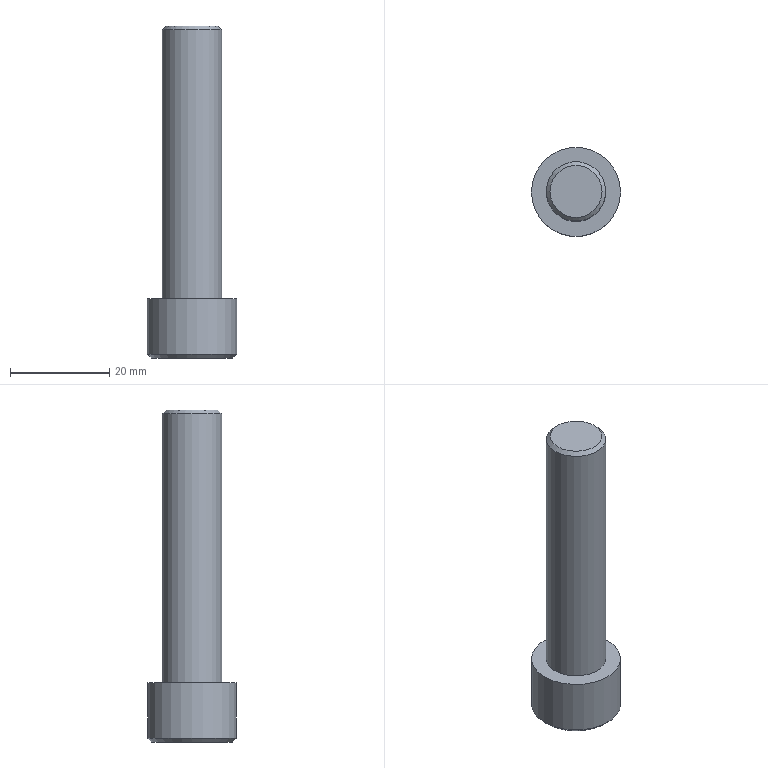Part | STEP file | M12.00-55.00 | 1 solid | 14 faces | box 18 x 18 x 67 mm | volume 8675 mm3 | plane 10 | cylinder 2 | cone 2 | commonest cylinder face diameters 12 x1 18 x1